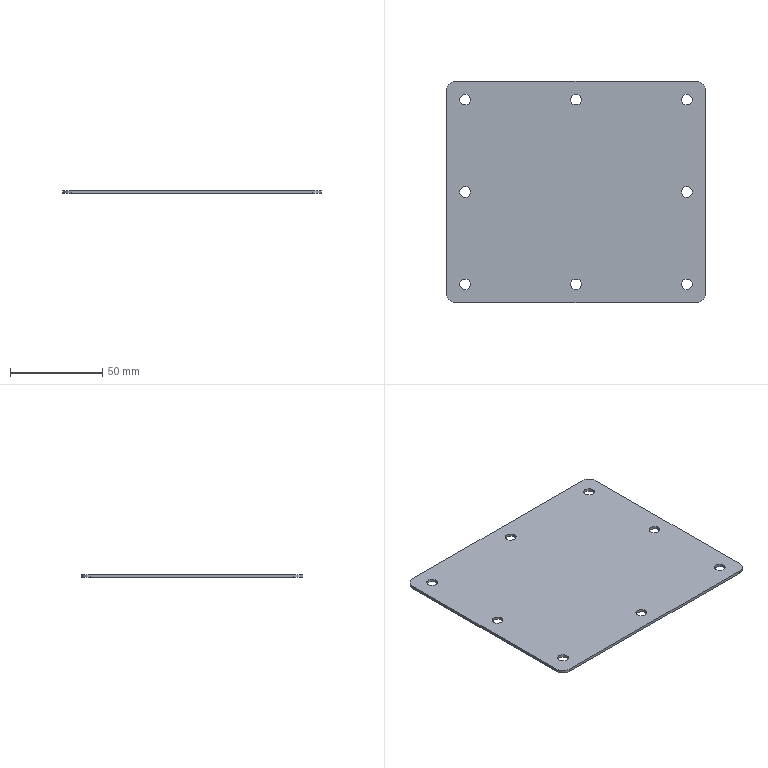Part | SolidWorks | features BreakCorner 1, FlatPattern 1, HoleWzd 1, SMBaseFlange 1, SheetMetal 1 | 1 solid | 26 faces | box 140 x 120 x 1.5 mm | volume 24851 mm3 | cylinder 20 | plane 6 | commonest cylinder face diameters 5.8 x16 10 x4
STEP:
#1=CARTESIAN_POINT('',(-62.9,50.,-1.5));
#2=VERTEX_POINT('',#1);
#3=CARTESIAN_POINT('',(-57.1,50.,-1.5));
#4=VERTEX_POINT('',#3);
#5=CARTESIAN_POINT('',(-60.,50.,-1.5));
#6=DIRECTION('',(0.,0.,1.));
#7=DIRECTION('',(1.,0.,0.));
#8=AXIS2_PLACEMENT_3D('',#5,#6,#7);
#9=CIRCLE('',#8,2.9);
#10=EDGE_CURVE('',#2,#4,#9,.T.);
#11=ORIENTED_EDGE('',*,*,#10,.F.);
#12=CARTESIAN_POINT('',(-62.9,50.,0.));
#13=VERTEX_POINT('',#12);
#14=CARTESIAN_POINT('',(-62.9,50.,0.));
#15=DIRECTION('',(0.,0.,1.));
#16=VECTOR('',#15,1000.);
#17=LINE('',#14,#16);
#18=EDGE_CURVE('',#2,#13,#17,.T.);
#19=ORIENTED_EDGE('',*,*,#18,.T.);
#20=CARTESIAN_POINT('',(-57.1,50.,0.));
#21=VERTEX_POINT('',#20);
#22=CARTESIAN_POINT('',(-60.,50.,0.));
#23=DIRECTION('',(0.,0.,1.));
#24=DIRECTION('',(1.,0.,0.));
#25=AXIS2_PLACEMENT_3D('',#22,#23,#24);
#26=CIRCLE('',#25,2.9);
#27=EDGE_CURVE('',#13,#21,#26,.T.);
#28=ORIENTED_EDGE('',*,*,#27,.T.);
#29=CARTESIAN_POINT('',(-57.1,50.,0.));
#30=DIRECTION('',(0.,0.,1.));
#31=VECTOR('',#30,1000.);
#32=LINE('',#29,#31);
#33=EDGE_CURVE('',#4,#21,#32,.T.);
#34=ORIENTED_EDGE('',*,*,#33,.F.);
#35=EDGE_LOOP('',(#11,#19,#28,#34));
#36=FACE_OUTER_BOUND('',#35,.T.);
#37=CARTESIAN_POINT('',(-60.,50.,0.));
#38=DIRECTION('',(0.,0.,1.));
#39=DIRECTION('',(1.,0.,0.));
#40=AXIS2_PLACEMENT_3D('',#37,#38,#39);
#41=CYLINDRICAL_SURFACE('',#40,2.9);
#42=ADVANCED_FACE('',(#36),#41,.F.);
#43=CARTESIAN_POINT('',(57.1,50.,-1.5));
#44=VERTEX_POINT('',#43);
#45=CARTESIAN_POINT('',(62.9,50.,-1.5));
#46=VERTEX_POINT('',#45);
#47=CARTESIAN_POINT('',(60.,50.,-1.5));
#48=DIRECTION('',(0.,0.,1.));
#49=DIRECTION('',(1.,0.,0.));
#50=AXIS2_PLACEMENT_3D('',#47,#48,#49);
#51=CIRCLE('',#50,2.9);
#52=EDGE_CURVE('',#44,#46,#51,.T.);
#53=ORIENTED_EDGE('',*,*,#52,.F.);
#54=CARTESIAN_POINT('',(57.1,50.,0.));
#55=VERTEX_POINT('',#54);
#56=CARTESIAN_POINT('',(57.1,50.,0.));
#57=DIRECTION('',(0.,0.,1.));
#58=VECTOR('',#57,1000.);
#59=LINE('',#56,#58);
#60=EDGE_CURVE('',#44,#55,#59,.T.);
#61=ORIENTED_EDGE('',*,*,#60,.T.);
#62=CARTESIAN_POINT('',(62.9,50.,0.));
#63=VERTEX_POINT('',#62);
#64=CARTESIAN_POINT('',(60.,50.,0.));
#65=DIRECTION('',(0.,0.,1.));
#66=DIRECTION('',(1.,0.,0.));
#67=AXIS2_PLACEMENT_3D('',#64,#65,#66);
#68=CIRCLE('',#67,2.9);
#69=EDGE_CURVE('',#55,#63,#68,.T.);
#70=ORIENTED_EDGE('',*,*,#69,.T.);
#71=CARTESIAN_POINT('',(62.9,50.,0.));
#72=DIRECTION('',(0.,0.,1.));
#73=VECTOR('',#72,1000.);
#74=LINE('',#71,#73);
#75=EDGE_CURVE('',#46,#63,#74,.T.);
#76=ORIENTED_EDGE('',*,*,#75,.F.);
#77=EDGE_LOOP('',(#53,#61,#70,#76));
#78=FACE_OUTER_BOUND('',#77,.T.);
#79=CARTESIAN_POINT('',(60.,50.,0.));
#80=DIRECTION('',(0.,0.,1.));
#81=DIRECTION('',(1.,0.,0.));
#82=AXIS2_PLACEMENT_3D('',#79,#80,#81);
#83=CYLINDRICAL_SURFACE('',#82,2.9);
#84=ADVANCED_FACE('',(#78),#83,.F.);
#85=CARTESIAN_POINT('',(-62.9,-50.,-1.5));
#86=VERTEX_POINT('',#85);
#87=CARTESIAN_POINT('',(-57.1,-50.,-1.5));
#88=VERTEX_POINT('',#87);
#89=CARTESIAN_POINT('',(-60.,-50.,-1.5));
#90=DIRECTION('',(0.,0.,1.));
#91=DIRECTION('',(1.,0.,0.));
#92=AXIS2_PLACEMENT_3D('',#89,#90,#91);
#93=CIRCLE('',#92,2.9);
#94=EDGE_CURVE('',#86,#88,#93,.T.);
#95=ORIENTED_EDGE('',*,*,#94,.F.);
#96=CARTESIAN_POINT('',(-62.9,-50.,0.));
#97=VERTEX_POINT('',#96);
#98=CARTESIAN_POINT('',(-62.9,-50.,0.));
#99=DIRECTION('',(0.,0.,1.));
#100=VECTOR('',#99,1000.);
#101=LINE('',#98,#100);
#102=EDGE_CURVE('',#86,#97,#101,.T.);
#103=ORIENTED_EDGE('',*,*,#102,.T.);
#104=CARTESIAN_POINT('',(-57.1,-50.,0.));
#105=VERTEX_POINT('',#104);
#106=CARTESIAN_POINT('',(-60.,-50.,0.));
#107=DIRECTION('',(0.,0.,1.));
#108=DIRECTION('',(1.,0.,0.));
#109=AXIS2_PLACEMENT_3D('',#106,#107,#108);
#110=CIRCLE('',#109,2.9);
#111=EDGE_CURVE('',#97,#105,#110,.T.);
#112=ORIENTED_EDGE('',*,*,#111,.T.);
#113=CARTESIAN_POINT('',(-57.1,-50.,0.));
#114=DIRECTION('',(0.,0.,1.));
#115=VECTOR('',#114,1000.);
#116=LINE('',#113,#115);
#117=EDGE_CURVE('',#88,#105,#116,.T.);
#118=ORIENTED_EDGE('',*,*,#117,.F.);
#119=EDGE_LOOP('',(#95,#103,#112,#118));
#120=FACE_OUTER_BOUND('',#119,.T.);
#121=CARTESIAN_POINT('',(-60.,-50.,0.));
#122=DIRECTION('',(0.,0.,1.));
#123=DIRECTION('',(1.,0.,0.));
#124=AXIS2_PLACEMENT_3D('',#121,#122,#123);
#125=CYLINDRICAL_SURFACE('',#124,2.9);
#126=ADVANCED_FACE('',(#120),#125,.F.);
#127=CARTESIAN_POINT('',(57.1,-50.,-1.5));
#128=VERTEX_POINT('',#127);
#129=CARTESIAN_POINT('',(62.9,-50.,-1.5));
#130=VERTEX_POINT('',#129);
#131=CARTESIAN_POINT('',(60.,-50.,-1.5));
#132=DIRECTION('',(0.,0.,1.));
#133=DIRECTION('',(1.,0.,0.));
#134=AXIS2_PLACEMENT_3D('',#131,#132,#133);
#135=CIRCLE('',#134,2.9);
#136=EDGE_CURVE('',#128,#130,#135,.T.);
#137=ORIENTED_EDGE('',*,*,#136,.F.);
#138=CARTESIAN_POINT('',(57.1,-50.,0.));
#139=VERTEX_POINT('',#138);
#140=CARTESIAN_POINT('',(57.1,-50.,0.));
#141=DIRECTION('',(0.,0.,1.));
#142=VECTOR('',#141,1000.);
#143=LINE('',#140,#142);
#144=EDGE_CURVE('',#128,#139,#143,.T.);
#145=ORIENTED_EDGE('',*,*,#144,.T.);
#146=CARTESIAN_POINT('',(62.9,-50.,0.));
#147=VERTEX_POINT('',#146);
#148=CARTESIAN_POINT('',(60.,-50.,0.));
#149=DIRECTION('',(0.,0.,1.));
#150=DIRECTION('',(1.,0.,0.));
#151=AXIS2_PLACEMENT_3D('',#148,#149,#150);
#152=CIRCLE('',#151,2.9);
#153=EDGE_CURVE('',#139,#147,#152,.T.);
#154=ORIENTED_EDGE('',*,*,#153,.T.);
#155=CARTESIAN_POINT('',(62.9,-50.,0.));
#156=DIRECTION('',(0.,0.,1.));
#157=VECTOR('',#156,1000.);
#158=LINE('',#155,#157);
#159=EDGE_CURVE('',#130,#147,#158,.T.);
#160=ORIENTED_EDGE('',*,*,#159,.F.);
#161=EDGE_LOOP('',(#137,#145,#154,#160));
#162=FACE_OUTER_BOUND('',#161,.T.);
#163=CARTESIAN_POINT('',(60.,-50.,0.));
#164=DIRECTION('',(0.,0.,1.));
#165=DIRECTION('',(1.,0.,0.));
#166=AXIS2_PLACEMENT_3D('',#163,#164,#165);
#167=CYLINDRICAL_SURFACE('',#166,2.9);
#168=ADVANCED_FACE('',(#162),#167,.F.);
#169=CARTESIAN_POINT('',(-62.9,0.,-1.5));
#170=VERTEX_POINT('',#169);
#171=CARTESIAN_POINT('',(-57.1,0.,-1.5));
#172=VERTEX_POINT('',#171);
#173=CARTESIAN_POINT('',(-60.,0.,-1.5));
#174=DIRECTION('',(0.,0.,1.));
#175=DIRECTION('',(1.,0.,0.));
#176=AXIS2_PLACEMENT_3D('',#173,#174,#175);
#177=CIRCLE('',#176,2.9);
#178=EDGE_CURVE('',#170,#172,#177,.T.);
#179=ORIENTED_EDGE('',*,*,#178,.F.);
#180=CARTESIAN_POINT('',(-62.9,0.,0.));
#181=VERTEX_POINT('',#180);
#182=CARTESIAN_POINT('',(-62.9,0.,0.));
#183=DIRECTION('',(0.,0.,1.));
#184=VECTOR('',#183,1000.);
#185=LINE('',#182,#184);
#186=EDGE_CURVE('',#170,#181,#185,.T.);
#187=ORIENTED_EDGE('',*,*,#186,.T.);
#188=CARTESIAN_POINT('',(-57.1,0.,0.));
#189=VERTEX_POINT('',#188);
#190=CARTESIAN_POINT('',(-60.,0.,0.));
#191=DIRECTION('',(0.,0.,1.));
#192=DIRECTION('',(1.,0.,0.));
#193=AXIS2_PLACEMENT_3D('',#190,#191,#192);
#194=CIRCLE('',#193,2.9);
#195=EDGE_CURVE('',#181,#189,#194,.T.);
#196=ORIENTED_EDGE('',*,*,#195,.T.);
#197=CARTESIAN_POINT('',(-57.1,0.,0.));
#198=DIRECTION('',(0.,0.,1.));
#199=VECTOR('',#198,1000.);
#200=LINE('',#197,#199);
#201=EDGE_CURVE('',#172,#189,#200,.T.);
#202=ORIENTED_EDGE('',*,*,#201,.F.);
#203=EDGE_LOOP('',(#179,#187,#196,#202));
#204=FACE_OUTER_BOUND('',#203,.T.);
#205=CARTESIAN_POINT('',(-60.,0.,0.));
#206=DIRECTION('',(0.,0.,1.));
#207=DIRECTION('',(1.,0.,0.));
#208=AXIS2_PLACEMENT_3D('',#205,#206,#207);
#209=CYLINDRICAL_SURFACE('',#208,2.9);
#210=ADVANCED_FACE('',(#204),#209,.F.);
#211=CARTESIAN_POINT('',(57.1,0.,-1.5));
#212=VERTEX_POINT('',#211);
#213=CARTESIAN_POINT('',(62.9,0.,-1.5));
#214=VERTEX_POINT('',#213);
#215=CARTESIAN_POINT('',(60.,0.,-1.5));
#216=DIRECTION('',(0.,0.,1.));
#217=DIRECTION('',(1.,0.,0.));
#218=AXIS2_PLACEMENT_3D('',#215,#216,#217);
#219=CIRCLE('',#218,2.9);
#220=EDGE_CURVE('',#212,#214,#219,.T.);
#221=ORIENTED_EDGE('',*,*,#220,.F.);
#222=CARTESIAN_POINT('',(57.1,0.,0.));
#223=VERTEX_POINT('',#222);
#224=CARTESIAN_POINT('',(57.1,0.,0.));
#225=DIRECTION('',(0.,0.,1.));
#226=VECTOR('',#225,1000.);
#227=LINE('',#224,#226);
#228=EDGE_CURVE('',#212,#223,#227,.T.);
#229=ORIENTED_EDGE('',*,*,#228,.T.);
#230=CARTESIAN_POINT('',(62.9,0.,0.));
#231=VERTEX_POINT('',#230);
#232=CARTESIAN_POINT('',(60.,0.,0.));
#233=DIRECTION('',(0.,0.,1.));
#234=DIRECTION('',(1.,0.,0.));
#235=AXIS2_PLACEMENT_3D('',#232,#233,#234);
#236=CIRCLE('',#235,2.9);
#237=EDGE_CURVE('',#223,#231,#236,.T.);
#238=ORIENTED_EDGE('',*,*,#237,.T.);
#239=CARTESIAN_POINT('',(62.9,0.,0.));
#240=DIRECTION('',(0.,0.,1.));
#241=VECTOR('',#240,1000.);
#242=LINE('',#239,#241);
#243=EDGE_CURVE('',#214,#231,#242,.T.);
#244=ORIENTED_EDGE('',*,*,#243,.F.);
#245=EDGE_LOOP('',(#221,#229,#238,#244));
#246=FACE_OUTER_BOUND('',#245,.T.);
#247=CARTESIAN_POINT('',(60.,0.,0.));
#248=DIRECTION('',(0.,0.,1.));
#249=DIRECTION('',(1.,0.,0.));
#250=AXIS2_PLACEMENT_3D('',#247,#248,#249);
#251=CYLINDRICAL_SURFACE('',#250,2.9);
#252=ADVANCED_FACE('',(#246),#251,.F.);
#253=CARTESIAN_POINT('',(-2.9,-50.,-1.5));
#254=VERTEX_POINT('',#253);
#255=CARTESIAN_POINT('',(2.9,-50.,-1.5));
#256=VERTEX_POINT('',#255);
#257=CARTESIAN_POINT('',(0.,-50.,-1.5));
#258=DIRECTION('',(0.,0.,1.));
#259=DIRECTION('',(1.,0.,0.));
#260=AXIS2_PLACEMENT_3D('',#257,#258,#259);
#261=CIRCLE('',#260,2.9);
#262=EDGE_CURVE('',#254,#256,#261,.T.);
#263=ORIENTED_EDGE('',*,*,#262,.F.);
#264=CARTESIAN_POINT('',(-2.9,-50.,0.));
#265=VERTEX_POINT('',#264);
#266=CARTESIAN_POINT('',(-2.9,-50.,0.));
#267=DIRECTION('',(0.,0.,1.));
#268=VECTOR('',#267,1000.);
#269=LINE('',#266,#268);
#270=EDGE_CURVE('',#254,#265,#269,.T.);
#271=ORIENTED_EDGE('',*,*,#270,.T.);
#272=CARTESIAN_POINT('',(2.9,-50.,0.));
#273=VERTEX_POINT('',#272);
#274=CARTESIAN_POINT('',(0.,-50.,0.));
#275=DIRECTION('',(0.,0.,1.));
#276=DIRECTION('',(1.,0.,0.));
#277=AXIS2_PLACEMENT_3D('',#274,#275,#276);
#278=CIRCLE('',#277,2.9);
#279=EDGE_CURVE('',#265,#273,#278,.T.);
#280=ORIENTED_EDGE('',*,*,#279,.T.);
#281=CARTESIAN_POINT('',(2.9,-50.,0.));
#282=DIRECTION('',(0.,0.,1.));
#283=VECTOR('',#282,1000.);
#284=LINE('',#281,#283);
#285=EDGE_CURVE('',#256,#273,#284,.T.);
#286=ORIENTED_EDGE('',*,*,#285,.F.);
#287=EDGE_LOOP('',(#263,#271,#280,#286));
#288=FACE_OUTER_BOUND('',#287,.T.);
#289=CARTESIAN_POINT('',(0.,-50.,0.));
#290=DIRECTION('',(0.,0.,1.));
#291=DIRECTION('',(1.,0.,0.));
#292=AXIS2_PLACEMENT_3D('',#289,#290,#291);
#293=CYLINDRICAL_SURFACE('',#292,2.9);
#294=ADVANCED_FACE('',(#288),#293,.F.);
#295=CARTESIAN_POINT('',(-2.9,50.,-1.5));
#296=VERTEX_POINT('',#295);
#297=CARTESIAN_POINT('',(2.9,50.,-1.5));
#298=VERTEX_POINT('',#297);
#299=CARTESIAN_POINT('',(0.,50.,-1.5));
#300=DIRECTION('',(0.,0.,1.));
#301=DIRECTION('',(1.,0.,0.));
#302=AXIS2_PLACEMENT_3D('',#299,#300,#301);
#303=CIRCLE('',#302,2.9);
#304=EDGE_CURVE('',#296,#298,#303,.T.);
#305=ORIENTED_EDGE('',*,*,#304,.F.);
#306=CARTESIAN_POINT('',(-2.9,50.,0.));
#307=VERTEX_POINT('',#306);
#308=CARTESIAN_POINT('',(-2.9,50.,0.));
#309=DIRECTION('',(0.,0.,1.));
#310=VECTOR('',#309,1000.);
#311=LINE('',#308,#310);
#312=EDGE_CURVE('',#296,#307,#311,.T.);
#313=ORIENTED_EDGE('',*,*,#312,.T.);
#314=CARTESIAN_POINT('',(2.9,50.,0.));
#315=VERTEX_POINT('',#314);
#316=CARTESIAN_POINT('',(0.,50.,0.));
#317=DIRECTION('',(0.,0.,1.));
#318=DIRECTION('',(1.,0.,0.));
#319=AXIS2_PLACEMENT_3D('',#316,#317,#318);
#320=CIRCLE('',#319,2.9);
#321=EDGE_CURVE('',#307,#315,#320,.T.);
#322=ORIENTED_EDGE('',*,*,#321,.T.);
#323=CARTESIAN_POINT('',(2.9,50.,0.));
#324=DIRECTION('',(0.,0.,1.));
#325=VECTOR('',#324,1000.);
#326=LINE('',#323,#325);
#327=EDGE_CURVE('',#298,#315,#326,.T.);
#328=ORIENTED_EDGE('',*,*,#327,.F.);
#329=EDGE_LOOP('',(#305,#313,#322,#328));
#330=FACE_OUTER_BOUND('',#329,.T.);
#331=CARTESIAN_POINT('',(0.,50.,0.));
#332=DIRECTION('',(0.,0.,1.));
#333=DIRECTION('',(1.,0.,0.));
#334=AXIS2_PLACEMENT_3D('',#331,#332,#333);
#335=CYLINDRICAL_SURFACE('',#334,2.9);
#336=ADVANCED_FACE('',(#330),#335,.F.);
#337=CARTESIAN_POINT('',(70.,-55.,0.));
#338=VERTEX_POINT('',#337);
#339=CARTESIAN_POINT('',(70.,55.,0.));
#340=VERTEX_POINT('',#339);
#341=CARTESIAN_POINT('',(70.,-60.,0.));
#342=DIRECTION('',(0.,1.,0.));
#343=VECTOR('',#342,1000.);
#344=LINE('',#341,#343);
#345=EDGE_CURVE('',#338,#340,#344,.T.);
#346=ORIENTED_EDGE('',*,*,#345,.F.);
#347=CARTESIAN_POINT('',(70.,-55.,-1.5));
#348=VERTEX_POINT('',#347);
#349=CARTESIAN_POINT('',(70.,-55.,-1.5));
#350=DIRECTION('',(0.,0.,-1.));
#351=VECTOR('',#350,1000.);
#352=LINE('',#349,#351);
#353=EDGE_CURVE('',#338,#348,#352,.T.);
#354=ORIENTED_EDGE('',*,*,#353,.T.);
#355=CARTESIAN_POINT('',(70.,55.,-1.5));
#356=VERTEX_POINT('',#355);
#357=CARTESIAN_POINT('',(70.,-60.,-1.5));
#358=DIRECTION('',(0.,1.,0.));
#359=VECTOR('',#358,1000.);
#360=LINE('',#357,#359);
#361=EDGE_CURVE('',#348,#356,#360,.T.);
#362=ORIENTED_EDGE('',*,*,#361,.T.);
#363=CARTESIAN_POINT('',(70.,55.,-1.5));
#364=DIRECTION('',(0.,0.,1.));
#365=VECTOR('',#364,1000.);
#366=LINE('',#363,#365);
#367=EDGE_CURVE('',#356,#340,#366,.T.);
#368=ORIENTED_EDGE('',*,*,#367,.T.);
#369=EDGE_LOOP('',(#346,#354,#362,#368));
#370=FACE_OUTER_BOUND('',#369,.T.);
#371=CARTESIAN_POINT('',(70.,-60.,-1.5));
#372=DIRECTION('',(1.,0.,0.));
#373=DIRECTION('',(0.,0.,-1.));
#374=AXIS2_PLACEMENT_3D('',#371,#372,#373);
#375=PLANE('',#374);
#376=ADVANCED_FACE('',(#370),#375,.T.);
#377=CARTESIAN_POINT('',(-65.,-60.,-1.5));
#378=VERTEX_POINT('',#377);
#379=CARTESIAN_POINT('',(65.,-60.,-1.5));
#380=VERTEX_POINT('',#379);
#381=CARTESIAN_POINT('',(-70.,-60.,-1.5));
#382=DIRECTION('',(1.,0.,0.));
#383=VECTOR('',#382,1000.);
#384=LINE('',#381,#383);
#385=EDGE_CURVE('',#378,#380,#384,.T.);
#386=ORIENTED_EDGE('',*,*,#385,.T.);
#387=CARTESIAN_POINT('',(65.,-60.,0.));
#388=VERTEX_POINT('',#387);
#389=CARTESIAN_POINT('',(65.,-60.,-1.5));
#390=DIRECTION('',(0.,0.,1.));
#391=VECTOR('',#390,1000.);
#392=LINE('',#389,#391);
#393=EDGE_CURVE('',#380,#388,#392,.T.);
#394=ORIENTED_EDGE('',*,*,#393,.T.);
#395=CARTESIAN_POINT('',(-65.,-60.,0.));
#396=VERTEX_POINT('',#395);
#397=CARTESIAN_POINT('',(-70.,-60.,0.));
#398=DIRECTION('',(1.,0.,0.));
#399=VECTOR('',#398,1000.);
#400=LINE('',#397,#399);
#401=EDGE_CURVE('',#396,#388,#400,.T.);
#402=ORIENTED_EDGE('',*,*,#401,.F.);
#403=CARTESIAN_POINT('',(-65.,-60.,-1.5));
#404=DIRECTION('',(0.,0.,-1.));
#405=VECTOR('',#404,1000.);
#406=LINE('',#403,#405);
#407=EDGE_CURVE('',#396,#378,#406,.T.);
#408=ORIENTED_EDGE('',*,*,#407,.T.);
#409=EDGE_LOOP('',(#386,#394,#402,#408));
#410=FACE_OUTER_BOUND('',#409,.T.);
#411=CARTESIAN_POINT('',(-70.,-60.,-1.5));
#412=DIRECTION('',(0.,-1.,0.));
#413=DIRECTION('',(0.,0.,-1.));
#414=AXIS2_PLACEMENT_3D('',#411,#412,#413);
#415=PLANE('',#414);
#416=ADVANCED_FACE('',(#410),#415,.T.);
#417=CARTESIAN_POINT('',(-70.,55.,-1.5));
#418=VERTEX_POINT('',#417);
#419=CARTESIAN_POINT('',(-70.,-55.,-1.5));
#420=VERTEX_POINT('',#419);
#421=CARTESIAN_POINT('',(-70.,-60.,-1.5));
#422=DIRECTION('',(0.,-1.,0.));
#423=VECTOR('',#422,1000.);
#424=LINE('',#421,#423);
#425=EDGE_CURVE('',#418,#420,#424,.T.);
#426=ORIENTED_EDGE('',*,*,#425,.T.);
#427=CARTESIAN_POINT('',(-70.,-55.,0.));
#428=VERTEX_POINT('',#427);
#429=CARTESIAN_POINT('',(-70.,-55.,-1.5));
#430=DIRECTION('',(0.,0.,1.));
#431=VECTOR('',#430,1000.);
#432=LINE('',#429,#431);
#433=EDGE_CURVE('',#420,#428,#432,.T.);
#434=ORIENTED_EDGE('',*,*,#433,.T.);
#435=CARTESIAN_POINT('',(-70.,55.,0.));
#436=VERTEX_POINT('',#435);
#437=CARTESIAN_POINT('',(-70.,-60.,0.));
#438=DIRECTION('',(0.,-1.,0.));
#439=VECTOR('',#438,1000.);
#440=LINE('',#437,#439);
#441=EDGE_CURVE('',#436,#428,#440,.T.);
#442=ORIENTED_EDGE('',*,*,#441,.F.);
#443=CARTESIAN_POINT('',(-70.,55.,-1.5));
#444=DIRECTION('',(0.,0.,-1.));
#445=VECTOR('',#444,1000.);
#446=LINE('',#443,#445);
#447=EDGE_CURVE('',#436,#418,#446,.T.);
#448=ORIENTED_EDGE('',*,*,#447,.T.);
#449=EDGE_LOOP('',(#426,#434,#442,#448));
#450=FACE_OUTER_BOUND('',#449,.T.);
#451=CARTESIAN_POINT('',(-70.,-60.,-1.5));
#452=DIRECTION('',(-1.,0.,0.));
#453=DIRECTION('',(0.,0.,1.));
#454=AXIS2_PLACEMENT_3D('',#451,#452,#453);
#455=PLANE('',#454);
#456=ADVANCED_FACE('',(#450),#455,.T.);
#457=CARTESIAN_POINT('',(65.,60.,-1.5));
#458=VERTEX_POINT('',#457);
#459=CARTESIAN_POINT('',(-65.,60.,-1.5));
#460=VERTEX_POINT('',#459);
#461=CARTESIAN_POINT('',(-70.,60.,-1.5));
#462=DIRECTION('',(-1.,0.,0.));
#463=VECTOR('',#462,1000.);
#464=LINE('',#461,#463);
#465=EDGE_CURVE('',#458,#460,#464,.T.);
#466=ORIENTED_EDGE('',*,*,#465,.T.);
#467=CARTESIAN_POINT('',(-65.,60.,0.));
#468=VERTEX_POINT('',#467);
#469=CARTESIAN_POINT('',(-65.,60.,-1.5));
#470=DIRECTION('',(0.,0.,1.));
#471=VECTOR('',#470,1000.);
#472=LINE('',#469,#471);
#473=EDGE_CURVE('',#460,#468,#472,.T.);
#474=ORIENTED_EDGE('',*,*,#473,.T.);
#475=CARTESIAN_POINT('',(65.,60.,0.));
#476=VERTEX_POINT('',#475);
#477=CARTESIAN_POINT('',(-70.,60.,0.));
#478=DIRECTION('',(-1.,0.,0.));
#479=VECTOR('',#478,1000.);
#480=LINE('',#477,#479);
#481=EDGE_CURVE('',#476,#468,#480,.T.);
#482=ORIENTED_EDGE('',*,*,#481,.F.);
#483=CARTESIAN_POINT('',(65.,60.,-1.5));
#484=DIRECTION('',(0.,0.,-1.));
#485=VECTOR('',#484,1000.);
#486=LINE('',#483,#485);
#487=EDGE_CURVE('',#476,#458,#486,.T.);
#488=ORIENTED_EDGE('',*,*,#487,.T.);
#489=EDGE_LOOP('',(#466,#474,#482,#488));
#490=FACE_OUTER_BOUND('',#489,.T.);
#491=CARTESIAN_POINT('',(-70.,60.,-1.5));
#492=DIRECTION('',(0.,1.,0.));
#493=DIRECTION('',(0.,0.,1.));
#494=AXIS2_PLACEMENT_3D('',#491,#492,#493);
#495=PLANE('',#494);
#496=ADVANCED_FACE('',(#490),#495,.T.);
#497=CARTESIAN_POINT('',(-60.,50.,-1.5));
#498=DIRECTION('',(0.,0.,1.));
#499=DIRECTION('',(1.,0.,0.));
#500=AXIS2_PLACEMENT_3D('',#497,#498,#499);
#501=CIRCLE('',#500,2.9);
#502=EDGE_CURVE('',#4,#2,#501,.T.);
#503=ORIENTED_EDGE('',*,*,#502,.T.);
#504=ORIENTED_EDGE('',*,*,#10,.T.);
#505=EDGE_LOOP('',(#503,#504));
#506=FACE_BOUND('',#505,.T.);
#507=CARTESIAN_POINT('',(60.,50.,-1.5));
#508=DIRECTION('',(0.,0.,1.));
#509=DIRECTION('',(1.,0.,0.));
#510=AXIS2_PLACEMENT_3D('',#507,#508,#509);
#511=CIRCLE('',#510,2.9);
#512=EDGE_CURVE('',#46,#44,#511,.T.);
#513=ORIENTED_EDGE('',*,*,#512,.T.);
#514=ORIENTED_EDGE('',*,*,#52,.T.);
#515=EDGE_LOOP('',(#513,#514));
#516=FACE_BOUND('',#515,.T.);
#517=CARTESIAN_POINT('',(-60.,-50.,-1.5));
#518=DIRECTION('',(0.,0.,1.));
#519=DIRECTION('',(1.,0.,0.));
#520=AXIS2_PLACEMENT_3D('',#517,#518,#519);
#521=CIRCLE('',#520,2.9);
#522=EDGE_CURVE('',#88,#86,#521,.T.);
#523=ORIENTED_EDGE('',*,*,#522,.T.);
#524=ORIENTED_EDGE('',*,*,#94,.T.);
#525=EDGE_LOOP('',(#523,#524));
#526=FACE_BOUND('',#525,.T.);
#527=CARTESIAN_POINT('',(60.,-50.,-1.5));
#528=DIRECTION('',(0.,0.,1.));
#529=DIRECTION('',(1.,0.,0.));
#530=AXIS2_PLACEMENT_3D('',#527,#528,#529);
#531=CIRCLE('',#530,2.9);
#532=EDGE_CURVE('',#130,#128,#531,.T.);
#533=ORIENTED_EDGE('',*,*,#532,.T.);
#534=ORIENTED_EDGE('',*,*,#136,.T.);
#535=EDGE_LOOP('',(#533,#534));
#536=FACE_BOUND('',#535,.T.);
#537=CARTESIAN_POINT('',(-60.,0.,-1.5));
#538=DIRECTION('',(0.,0.,1.));
#539=DIRECTION('',(1.,0.,0.));
#540=AXIS2_PLACEMENT_3D('',#537,#538,#539);
#541=CIRCLE('',#540,2.9);
#542=EDGE_CURVE('',#172,#170,#541,.T.);
#543=ORIENTED_EDGE('',*,*,#542,.T.);
#544=ORIENTED_EDGE('',*,*,#178,.T.);
#545=EDGE_LOOP('',(#543,#544));
#546=FACE_BOUND('',#545,.T.);
#547=CARTESIAN_POINT('',(60.,0.,-1.5));
#548=DIRECTION('',(0.,0.,1.));
#549=DIRECTION('',(1.,0.,0.));
#550=AXIS2_PLACEMENT_3D('',#547,#548,#549);
#551=CIRCLE('',#550,2.9);
#552=EDGE_CURVE('',#214,#212,#551,.T.);
#553=ORIENTED_EDGE('',*,*,#552,.T.);
#554=ORIENTED_EDGE('',*,*,#220,.T.);
#555=EDGE_LOOP('',(#553,#554));
#556=FACE_BOUND('',#555,.T.);
#557=CARTESIAN_POINT('',(0.,-50.,-1.5));
#558=DIRECTION('',(0.,0.,1.));
#559=DIRECTION('',(1.,0.,0.));
#560=AXIS2_PLACEMENT_3D('',#557,#558,#559);
#561=CIRCLE('',#560,2.9);
#562=EDGE_CURVE('',#256,#254,#561,.T.);
#563=ORIENTED_EDGE('',*,*,#562,.T.);
#564=ORIENTED_EDGE('',*,*,#262,.T.);
#565=EDGE_LOOP('',(#563,#564));
#566=FACE_BOUND('',#565,.T.);
#567=CARTESIAN_POINT('',(0.,50.,-1.5));
#568=DIRECTION('',(0.,0.,1.));
#569=DIRECTION('',(1.,0.,0.));
#570=AXIS2_PLACEMENT_3D('',#567,#568,#569);
#571=CIRCLE('',#570,2.9);
#572=EDGE_CURVE('',#298,#296,#571,.T.);
#573=ORIENTED_EDGE('',*,*,#572,.T.);
#574=ORIENTED_EDGE('',*,*,#304,.T.);
#575=EDGE_LOOP('',(#573,#574));
#576=FACE_BOUND('',#575,.T.);
#577=ORIENTED_EDGE('',*,*,#361,.F.);
#578=CARTESIAN_POINT('',(65.,-55.,-1.5));
#579=DIRECTION('',(0.,0.,-1.));
#580=DIRECTION('',(-1.,0.,0.));
#581=AXIS2_PLACEMENT_3D('',#578,#579,#580);
#582=CIRCLE('',#581,5.);
#583=EDGE_CURVE('',#348,#380,#582,.T.);
#584=ORIENTED_EDGE('',*,*,#583,.T.);
#585=ORIENTED_EDGE('',*,*,#385,.F.);
#586=CARTESIAN_POINT('',(-65.,-55.,-1.5));
#587=DIRECTION('',(0.,0.,-1.));
#588=DIRECTION('',(-1.,0.,0.));
#589=AXIS2_PLACEMENT_3D('',#586,#587,#588);
#590=CIRCLE('',#589,5.);
#591=EDGE_CURVE('',#378,#420,#590,.T.);
#592=ORIENTED_EDGE('',*,*,#591,.T.);
#593=ORIENTED_EDGE('',*,*,#425,.F.);
#594=CARTESIAN_POINT('',(-65.,55.,-1.5));
#595=DIRECTION('',(0.,0.,-1.));
#596=DIRECTION('',(-1.,0.,0.));
#597=AXIS2_PLACEMENT_3D('',#594,#595,#596);
#598=CIRCLE('',#597,5.);
#599=EDGE_CURVE('',#418,#460,#598,.T.);
#600=ORIENTED_EDGE('',*,*,#599,.T.);
#601=ORIENTED_EDGE('',*,*,#465,.F.);
#602=CARTESIAN_POINT('',(65.,55.,-1.5));
#603=DIRECTION('',(0.,0.,-1.));
#604=DIRECTION('',(-1.,0.,0.));
#605=AXIS2_PLACEMENT_3D('',#602,#603,#604);
#606=CIRCLE('',#605,5.);
#607=EDGE_CURVE('',#458,#356,#606,.T.);
#608=ORIENTED_EDGE('',*,*,#607,.T.);
#609=EDGE_LOOP('',(#577,#584,#585,#592,#593,#600,#601,#608));
#610=FACE_OUTER_BOUND('',#609,.T.);
#611=CARTESIAN_POINT('',(0.,0.,-1.5));
#612=DIRECTION('',(0.,0.,-1.));
#613=DIRECTION('',(-1.,0.,0.));
#614=AXIS2_PLACEMENT_3D('',#611,#612,#613);
#615=PLANE('',#614);
#616=ADVANCED_FACE('',(#506,#516,#526,#536,#546,#556,#566,#576,#610),#615,.T.);
#617=CARTESIAN_POINT('',(-60.,50.,0.));
#618=DIRECTION('',(0.,0.,1.));
#619=DIRECTION('',(1.,0.,0.));
#620=AXIS2_PLACEMENT_3D('',#617,#618,#619);
#621=CIRCLE('',#620,2.9);
#622=EDGE_CURVE('',#21,#13,#621,.T.);
#623=ORIENTED_EDGE('',*,*,#622,.F.);
#624=ORIENTED_EDGE('',*,*,#27,.F.);
#625=EDGE_LOOP('',(#623,#624));
#626=FACE_BOUND('',#625,.T.);
#627=CARTESIAN_POINT('',(60.,50.,0.));
#628=DIRECTION('',(0.,0.,1.));
#629=DIRECTION('',(1.,0.,0.));
#630=AXIS2_PLACEMENT_3D('',#627,#628,#629);
#631=CIRCLE('',#630,2.9);
#632=EDGE_CURVE('',#63,#55,#631,.T.);
#633=ORIENTED_EDGE('',*,*,#632,.F.);
#634=ORIENTED_EDGE('',*,*,#69,.F.);
#635=EDGE_LOOP('',(#633,#634));
#636=FACE_BOUND('',#635,.T.);
#637=CARTESIAN_POINT('',(-60.,-50.,0.));
#638=DIRECTION('',(0.,0.,1.));
#639=DIRECTION('',(1.,0.,0.));
#640=AXIS2_PLACEMENT_3D('',#637,#638,#639);
#641=CIRCLE('',#640,2.9);
#642=EDGE_CURVE('',#105,#97,#641,.T.);
#643=ORIENTED_EDGE('',*,*,#642,.F.);
#644=ORIENTED_EDGE('',*,*,#111,.F.);
#645=EDGE_LOOP('',(#643,#644));
#646=FACE_BOUND('',#645,.T.);
#647=CARTESIAN_POINT('',(60.,-50.,0.));
#648=DIRECTION('',(0.,0.,1.));
#649=DIRECTION('',(1.,0.,0.));
#650=AXIS2_PLACEMENT_3D('',#647,#648,#649);
#651=CIRCLE('',#650,2.9);
#652=EDGE_CURVE('',#147,#139,#651,.T.);
#653=ORIENTED_EDGE('',*,*,#652,.F.);
#654=ORIENTED_EDGE('',*,*,#153,.F.);
#655=EDGE_LOOP('',(#653,#654));
#656=FACE_BOUND('',#655,.T.);
#657=CARTESIAN_POINT('',(-60.,0.,0.));
#658=DIRECTION('',(0.,0.,1.));
#659=DIRECTION('',(1.,0.,0.));
#660=AXIS2_PLACEMENT_3D('',#657,#658,#659);
#661=CIRCLE('',#660,2.9);
#662=EDGE_CURVE('',#189,#181,#661,.T.);
#663=ORIENTED_EDGE('',*,*,#662,.F.);
#664=ORIENTED_EDGE('',*,*,#195,.F.);
#665=EDGE_LOOP('',(#663,#664));
#666=FACE_BOUND('',#665,.T.);
#667=CARTESIAN_POINT('',(60.,0.,0.));
#668=DIRECTION('',(0.,0.,1.));
#669=DIRECTION('',(1.,0.,0.));
#670=AXIS2_PLACEMENT_3D('',#667,#668,#669);
#671=CIRCLE('',#670,2.9);
#672=EDGE_CURVE('',#231,#223,#671,.T.);
#673=ORIENTED_EDGE('',*,*,#672,.F.);
#674=ORIENTED_EDGE('',*,*,#237,.F.);
#675=EDGE_LOOP('',(#673,#674));
#676=FACE_BOUND('',#675,.T.);
#677=CARTESIAN_POINT('',(0.,-50.,0.));
#678=DIRECTION('',(0.,0.,1.));
#679=DIRECTION('',(1.,0.,0.));
#680=AXIS2_PLACEMENT_3D('',#677,#678,#679);
#681=CIRCLE('',#680,2.9);
#682=EDGE_CURVE('',#273,#265,#681,.T.);
#683=ORIENTED_EDGE('',*,*,#682,.F.);
#684=ORIENTED_EDGE('',*,*,#279,.F.);
#685=EDGE_LOOP('',(#683,#684));
#686=FACE_BOUND('',#685,.T.);
#687=CARTESIAN_POINT('',(0.,50.,0.));
#688=DIRECTION('',(0.,0.,1.));
#689=DIRECTION('',(1.,0.,0.));
#690=AXIS2_PLACEMENT_3D('',#687,#688,#689);
#691=CIRCLE('',#690,2.9);
#692=EDGE_CURVE('',#315,#307,#691,.T.);
#693=ORIENTED_EDGE('',*,*,#692,.F.);
#694=ORIENTED_EDGE('',*,*,#321,.F.);
#695=EDGE_LOOP('',(#693,#694));
#696=FACE_BOUND('',#695,.T.);
#697=ORIENTED_EDGE('',*,*,#401,.T.);
#698=CARTESIAN_POINT('',(65.,-55.,0.));
#699=DIRECTION('',(0.,0.,1.));
#700=DIRECTION('',(-1.,0.,0.));
#701=AXIS2_PLACEMENT_3D('',#698,#699,#700);
#702=CIRCLE('',#701,5.);
#703=EDGE_CURVE('',#388,#338,#702,.T.);
#704=ORIENTED_EDGE('',*,*,#703,.T.);
#705=ORIENTED_EDGE('',*,*,#345,.T.);
#706=CARTESIAN_POINT('',(65.,55.,0.));
#707=DIRECTION('',(0.,0.,1.));
#708=DIRECTION('',(-1.,0.,0.));
#709=AXIS2_PLACEMENT_3D('',#706,#707,#708);
#710=CIRCLE('',#709,5.);
#711=EDGE_CURVE('',#340,#476,#710,.T.);
#712=ORIENTED_EDGE('',*,*,#711,.T.);
#713=ORIENTED_EDGE('',*,*,#481,.T.);
#714=CARTESIAN_POINT('',(-65.,55.,0.));
#715=DIRECTION('',(0.,0.,1.));
#716=DIRECTION('',(-1.,0.,0.));
#717=AXIS2_PLACEMENT_3D('',#714,#715,#716);
#718=CIRCLE('',#717,5.);
#719=EDGE_CURVE('',#468,#436,#718,.T.);
#720=ORIENTED_EDGE('',*,*,#719,.T.);
#721=ORIENTED_EDGE('',*,*,#441,.T.);
#722=CARTESIAN_POINT('',(-65.,-55.,0.));
#723=DIRECTION('',(0.,0.,1.));
#724=DIRECTION('',(-1.,0.,0.));
#725=AXIS2_PLACEMENT_3D('',#722,#723,#724);
#726=CIRCLE('',#725,5.);
#727=EDGE_CURVE('',#428,#396,#726,.T.);
#728=ORIENTED_EDGE('',*,*,#727,.T.);
#729=EDGE_LOOP('',(#697,#704,#705,#712,#713,#720,#721,#728));
#730=FACE_OUTER_BOUND('',#729,.T.);
#731=CARTESIAN_POINT('',(0.,0.,0.));
#732=DIRECTION('',(0.,0.,-1.));
#733=DIRECTION('',(-1.,0.,0.));
#734=AXIS2_PLACEMENT_3D('',#731,#732,#733);
#735=PLANE('',#734);
#736=ADVANCED_FACE('',(#626,#636,#646,#656,#666,#676,#686,#696,#730),#735,.F.);
#737=ORIENTED_EDGE('',*,*,#312,.F.);
#738=ORIENTED_EDGE('',*,*,#572,.F.);
#739=ORIENTED_EDGE('',*,*,#327,.T.);
#740=ORIENTED_EDGE('',*,*,#692,.T.);
#741=EDGE_LOOP('',(#737,#738,#739,#740));
#742=FACE_OUTER_BOUND('',#741,.T.);
#743=CARTESIAN_POINT('',(0.,50.,0.));
#744=DIRECTION('',(0.,0.,1.));
#745=DIRECTION('',(1.,0.,0.));
#746=AXIS2_PLACEMENT_3D('',#743,#744,#745);
#747=CYLINDRICAL_SURFACE('',#746,2.9);
#748=ADVANCED_FACE('',(#742),#747,.F.);
#749=ORIENTED_EDGE('',*,*,#270,.F.);
#750=ORIENTED_EDGE('',*,*,#562,.F.);
#751=ORIENTED_EDGE('',*,*,#285,.T.);
#752=ORIENTED_EDGE('',*,*,#682,.T.);
#753=EDGE_LOOP('',(#749,#750,#751,#752));
#754=FACE_OUTER_BOUND('',#753,.T.);
#755=CARTESIAN_POINT('',(0.,-50.,0.));
#756=DIRECTION('',(0.,0.,1.));
#757=DIRECTION('',(1.,0.,0.));
#758=AXIS2_PLACEMENT_3D('',#755,#756,#757);
#759=CYLINDRICAL_SURFACE('',#758,2.9);
#760=ADVANCED_FACE('',(#754),#759,.F.);
#761=ORIENTED_EDGE('',*,*,#228,.F.);
#762=ORIENTED_EDGE('',*,*,#552,.F.);
#763=ORIENTED_EDGE('',*,*,#243,.T.);
#764=ORIENTED_EDGE('',*,*,#672,.T.);
#765=EDGE_LOOP('',(#761,#762,#763,#764));
#766=FACE_OUTER_BOUND('',#765,.T.);
#767=CARTESIAN_POINT('',(60.,0.,0.));
#768=DIRECTION('',(0.,0.,1.));
#769=DIRECTION('',(1.,0.,0.));
#770=AXIS2_PLACEMENT_3D('',#767,#768,#769);
#771=CYLINDRICAL_SURFACE('',#770,2.9);
#772=ADVANCED_FACE('',(#766),#771,.F.);
#773=ORIENTED_EDGE('',*,*,#186,.F.);
#774=ORIENTED_EDGE('',*,*,#542,.F.);
#775=ORIENTED_EDGE('',*,*,#201,.T.);
#776=ORIENTED_EDGE('',*,*,#662,.T.);
#777=EDGE_LOOP('',(#773,#774,#775,#776));
#778=FACE_OUTER_BOUND('',#777,.T.);
#779=CARTESIAN_POINT('',(-60.,0.,0.));
#780=DIRECTION('',(0.,0.,1.));
#781=DIRECTION('',(1.,0.,0.));
#782=AXIS2_PLACEMENT_3D('',#779,#780,#781);
#783=CYLINDRICAL_SURFACE('',#782,2.9);
#784=ADVANCED_FACE('',(#778),#783,.F.);
#785=ORIENTED_EDGE('',*,*,#144,.F.);
#786=ORIENTED_EDGE('',*,*,#532,.F.);
#787=ORIENTED_EDGE('',*,*,#159,.T.);
#788=ORIENTED_EDGE('',*,*,#652,.T.);
#789=EDGE_LOOP('',(#785,#786,#787,#788));
#790=FACE_OUTER_BOUND('',#789,.T.);
#791=CARTESIAN_POINT('',(60.,-50.,0.));
#792=DIRECTION('',(0.,0.,1.));
#793=DIRECTION('',(1.,0.,0.));
#794=AXIS2_PLACEMENT_3D('',#791,#792,#793);
#795=CYLINDRICAL_SURFACE('',#794,2.9);
#796=ADVANCED_FACE('',(#790),#795,.F.);
#797=ORIENTED_EDGE('',*,*,#102,.F.);
#798=ORIENTED_EDGE('',*,*,#522,.F.);
#799=ORIENTED_EDGE('',*,*,#117,.T.);
#800=ORIENTED_EDGE('',*,*,#642,.T.);
#801=EDGE_LOOP('',(#797,#798,#799,#800));
#802=FACE_OUTER_BOUND('',#801,.T.);
#803=CARTESIAN_POINT('',(-60.,-50.,0.));
#804=DIRECTION('',(0.,0.,1.));
#805=DIRECTION('',(1.,0.,0.));
#806=AXIS2_PLACEMENT_3D('',#803,#804,#805);
#807=CYLINDRICAL_SURFACE('',#806,2.9);
#808=ADVANCED_FACE('',(#802),#807,.F.);
#809=ORIENTED_EDGE('',*,*,#60,.F.);
#810=ORIENTED_EDGE('',*,*,#512,.F.);
#811=ORIENTED_EDGE('',*,*,#75,.T.);
#812=ORIENTED_EDGE('',*,*,#632,.T.);
#813=EDGE_LOOP('',(#809,#810,#811,#812));
#814=FACE_OUTER_BOUND('',#813,.T.);
#815=CARTESIAN_POINT('',(60.,50.,0.));
#816=DIRECTION('',(0.,0.,1.));
#817=DIRECTION('',(1.,0.,0.));
#818=AXIS2_PLACEMENT_3D('',#815,#816,#817);
#819=CYLINDRICAL_SURFACE('',#818,2.9);
#820=ADVANCED_FACE('',(#814),#819,.F.);
#821=ORIENTED_EDGE('',*,*,#18,.F.);
#822=ORIENTED_EDGE('',*,*,#502,.F.);
#823=ORIENTED_EDGE('',*,*,#33,.T.);
#824=ORIENTED_EDGE('',*,*,#622,.T.);
#825=EDGE_LOOP('',(#821,#822,#823,#824));
#826=FACE_OUTER_BOUND('',#825,.T.);
#827=CARTESIAN_POINT('',(-60.,50.,0.));
#828=DIRECTION('',(0.,0.,1.));
#829=DIRECTION('',(1.,0.,0.));
#830=AXIS2_PLACEMENT_3D('',#827,#828,#829);
#831=CYLINDRICAL_SURFACE('',#830,2.9);
#832=ADVANCED_FACE('',(#826),#831,.F.);
#833=ORIENTED_EDGE('',*,*,#583,.F.);
#834=ORIENTED_EDGE('',*,*,#353,.F.);
#835=ORIENTED_EDGE('',*,*,#703,.F.);
#836=ORIENTED_EDGE('',*,*,#393,.F.);
#837=EDGE_LOOP('',(#833,#834,#835,#836));
#838=FACE_OUTER_BOUND('',#837,.T.);
#839=CARTESIAN_POINT('',(65.,-55.,-1.5));
#840=DIRECTION('',(0.,0.,1.));
#841=DIRECTION('',(1.,0.,0.));
#842=AXIS2_PLACEMENT_3D('',#839,#840,#841);
#843=CYLINDRICAL_SURFACE('',#842,5.);
#844=ADVANCED_FACE('',(#838),#843,.T.);
#845=ORIENTED_EDGE('',*,*,#591,.F.);
#846=ORIENTED_EDGE('',*,*,#407,.F.);
#847=ORIENTED_EDGE('',*,*,#727,.F.);
#848=ORIENTED_EDGE('',*,*,#433,.F.);
#849=EDGE_LOOP('',(#845,#846,#847,#848));
#850=FACE_OUTER_BOUND('',#849,.T.);
#851=CARTESIAN_POINT('',(-65.,-55.,-1.5));
#852=DIRECTION('',(0.,0.,1.));
#853=DIRECTION('',(1.,0.,0.));
#854=AXIS2_PLACEMENT_3D('',#851,#852,#853);
#855=CYLINDRICAL_SURFACE('',#854,5.);
#856=ADVANCED_FACE('',(#850),#855,.T.);
#857=ORIENTED_EDGE('',*,*,#599,.F.);
#858=ORIENTED_EDGE('',*,*,#447,.F.);
#859=ORIENTED_EDGE('',*,*,#719,.F.);
#860=ORIENTED_EDGE('',*,*,#473,.F.);
#861=EDGE_LOOP('',(#857,#858,#859,#860));
#862=FACE_OUTER_BOUND('',#861,.T.);
#863=CARTESIAN_POINT('',(-65.,55.,-1.5));
#864=DIRECTION('',(0.,0.,1.));
#865=DIRECTION('',(1.,0.,0.));
#866=AXIS2_PLACEMENT_3D('',#863,#864,#865);
#867=CYLINDRICAL_SURFACE('',#866,5.);
#868=ADVANCED_FACE('',(#862),#867,.T.);
#869=ORIENTED_EDGE('',*,*,#607,.F.);
#870=ORIENTED_EDGE('',*,*,#487,.F.);
#871=ORIENTED_EDGE('',*,*,#711,.F.);
#872=ORIENTED_EDGE('',*,*,#367,.F.);
#873=EDGE_LOOP('',(#869,#870,#871,#872));
#874=FACE_OUTER_BOUND('',#873,.T.);
#875=CARTESIAN_POINT('',(65.,55.,-1.5));
#876=DIRECTION('',(0.,0.,1.));
#877=DIRECTION('',(1.,0.,0.));
#878=AXIS2_PLACEMENT_3D('',#875,#876,#877);
#879=CYLINDRICAL_SURFACE('',#878,5.);
#880=ADVANCED_FACE('',(#874),#879,.T.);
#881=CLOSED_SHELL('',(#42,#84,#126,#168,#210,#252,#294,#336,#376,#416,#456,#496,#616,#736,#748,#760,#772,#784,#796,#808,#820,#832,#844,#856,#868,#880));
#882=MANIFOLD_SOLID_BREP('',#881);
#883=CARTESIAN_POINT('',(0.,0.,0.));
#884=DIRECTION('',(0.,0.,1.));
#885=DIRECTION('',(1.,0.,0.));
#886=AXIS2_PLACEMENT_3D('',#883,#884,#885);
#887=(LENGTH_UNIT()NAMED_UNIT(*)SI_UNIT(.MILLI.,.METRE.));
#888=UNCERTAINTY_MEASURE_WITH_UNIT(LENGTH_MEASURE(0.00001),#887,'','');
#889=(NAMED_UNIT(*)PLANE_ANGLE_UNIT()SI_UNIT($,.RADIAN.));
#890=(NAMED_UNIT(*)SI_UNIT($,.STERADIAN.)SOLID_ANGLE_UNIT());
#891=(GEOMETRIC_REPRESENTATION_CONTEXT(3)GLOBAL_UNCERTAINTY_ASSIGNED_CONTEXT((#888))GLOBAL_UNIT_ASSIGNED_CONTEXT((#887,#889,#890))REPRESENTATION_CONTEXT('',''));
#892=ADVANCED_BREP_SHAPE_REPRESENTATION('',(#882,#886),#891);